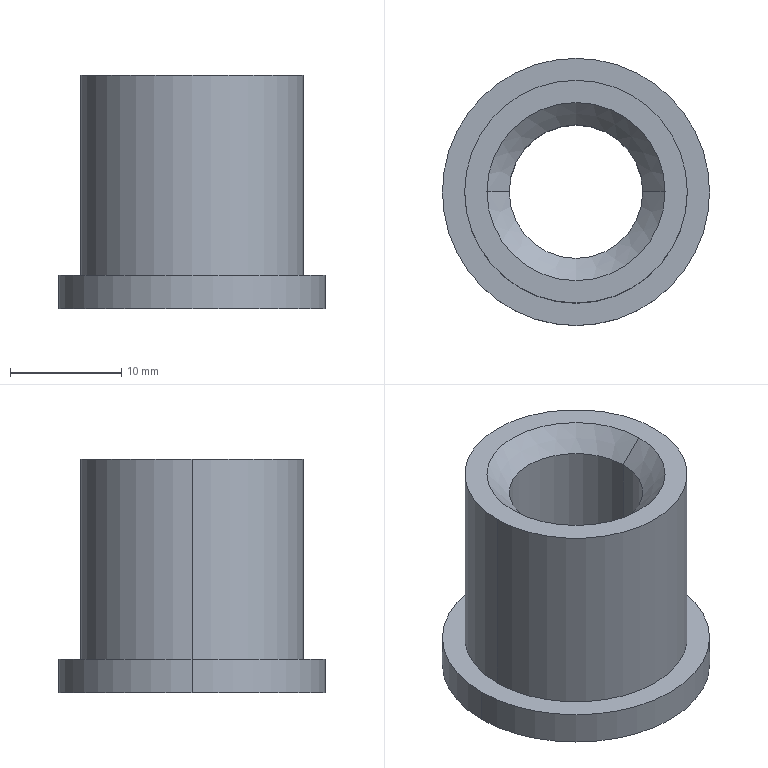Part | SolidWorks | features ICE 2, Chamfer 1, Extrusion 1 | 1 solid | 11 faces | box 24 x 24 x 21 mm | volume 4553 mm3 | cylinder 6 | plane 3 | cone 2 | commonest cylinder face diameters 12 x2 20 x2 24 x2
STEP:
#1=CARTESIAN_POINT('',(-6.,0.,19.));
#2=VERTEX_POINT('',#1);
#3=CARTESIAN_POINT('',(6.,0.,19.));
#4=VERTEX_POINT('',#3);
#5=CARTESIAN_POINT('',(0.,0.,19.));
#6=DIRECTION('',(0.,0.,1.));
#7=DIRECTION('',(1.,0.,0.));
#8=AXIS2_PLACEMENT_3D('',#5,#6,#7);
#9=CIRCLE('',#8,6.);
#10=EDGE_CURVE('',#2,#4,#9,.T.);
#11=ORIENTED_EDGE('',*,*,#10,.F.);
#12=CARTESIAN_POINT('',(-8.,0.,21.));
#13=VERTEX_POINT('',#12);
#14=CARTESIAN_POINT('',(-6.,0.,19.));
#15=DIRECTION('',(-0.7071,0.,0.7071));
#16=VECTOR('',#15,1000.);
#17=LINE('',#14,#16);
#18=EDGE_CURVE('',#2,#13,#17,.T.);
#19=ORIENTED_EDGE('',*,*,#18,.T.);
#20=CARTESIAN_POINT('',(8.,0.,21.));
#21=VERTEX_POINT('',#20);
#22=CARTESIAN_POINT('',(0.,0.,21.));
#23=DIRECTION('',(0.,0.,-1.));
#24=DIRECTION('',(1.,0.,0.));
#25=AXIS2_PLACEMENT_3D('',#22,#23,#24);
#26=CIRCLE('',#25,8.);
#27=EDGE_CURVE('',#21,#13,#26,.T.);
#28=ORIENTED_EDGE('',*,*,#27,.F.);
#29=CARTESIAN_POINT('',(6.,0.,19.));
#30=DIRECTION('',(0.7071,0.,0.7071));
#31=VECTOR('',#30,1000.);
#32=LINE('',#29,#31);
#33=EDGE_CURVE('',#4,#21,#32,.T.);
#34=ORIENTED_EDGE('',*,*,#33,.F.);
#35=EDGE_LOOP('',(#11,#19,#28,#34));
#36=FACE_OUTER_BOUND('',#35,.T.);
#37=CARTESIAN_POINT('',(0.,0.,19.));
#38=DIRECTION('',(0.,0.,1.));
#39=DIRECTION('',(1.,0.,0.));
#40=AXIS2_PLACEMENT_3D('',#37,#38,#39);
#41=CONICAL_SURFACE('',#40,6.,0.7854);
#42=ADVANCED_FACE('',(#36),#41,.F.);
#43=CARTESIAN_POINT('',(-6.,0.,0.));
#44=VERTEX_POINT('',#43);
#45=CARTESIAN_POINT('',(6.,0.,0.));
#46=VERTEX_POINT('',#45);
#47=CARTESIAN_POINT('',(0.,0.,0.));
#48=DIRECTION('',(0.,0.,1.));
#49=DIRECTION('',(1.,0.,0.));
#50=AXIS2_PLACEMENT_3D('',#47,#48,#49);
#51=CIRCLE('',#50,6.);
#52=EDGE_CURVE('',#44,#46,#51,.T.);
#53=ORIENTED_EDGE('',*,*,#52,.F.);
#54=CARTESIAN_POINT('',(-6.,0.,-5.));
#55=DIRECTION('',(0.,0.,1.));
#56=VECTOR('',#55,1000.);
#57=LINE('',#54,#56);
#58=EDGE_CURVE('',#44,#2,#57,.T.);
#59=ORIENTED_EDGE('',*,*,#58,.T.);
#60=ORIENTED_EDGE('',*,*,#10,.T.);
#61=CARTESIAN_POINT('',(6.,0.,-5.));
#62=DIRECTION('',(0.,0.,1.));
#63=VECTOR('',#62,1000.);
#64=LINE('',#61,#63);
#65=EDGE_CURVE('',#46,#4,#64,.T.);
#66=ORIENTED_EDGE('',*,*,#65,.F.);
#67=EDGE_LOOP('',(#53,#59,#60,#66));
#68=FACE_OUTER_BOUND('',#67,.T.);
#69=CARTESIAN_POINT('',(0.,0.,-5.));
#70=DIRECTION('',(0.,0.,1.));
#71=DIRECTION('',(1.,0.,0.));
#72=AXIS2_PLACEMENT_3D('',#69,#70,#71);
#73=CYLINDRICAL_SURFACE('',#72,6.);
#74=ADVANCED_FACE('',(#68),#73,.F.);
#75=CARTESIAN_POINT('',(10.,0.,21.));
#76=VERTEX_POINT('',#75);
#77=CARTESIAN_POINT('',(-10.,0.,21.));
#78=VERTEX_POINT('',#77);
#79=CARTESIAN_POINT('',(0.,0.,21.));
#80=DIRECTION('',(0.,0.,1.));
#81=DIRECTION('',(1.,0.,0.));
#82=AXIS2_PLACEMENT_3D('',#79,#80,#81);
#83=CIRCLE('',#82,10.);
#84=EDGE_CURVE('',#76,#78,#83,.T.);
#85=ORIENTED_EDGE('',*,*,#84,.F.);
#86=CARTESIAN_POINT('',(10.,0.,3.));
#87=VERTEX_POINT('',#86);
#88=CARTESIAN_POINT('',(10.,0.,21.));
#89=DIRECTION('',(0.,0.,-1.));
#90=VECTOR('',#89,1000.);
#91=LINE('',#88,#90);
#92=EDGE_CURVE('',#76,#87,#91,.T.);
#93=ORIENTED_EDGE('',*,*,#92,.T.);
#94=CARTESIAN_POINT('',(-10.,0.,3.));
#95=VERTEX_POINT('',#94);
#96=CARTESIAN_POINT('',(0.,0.,3.));
#97=DIRECTION('',(0.,0.,1.));
#98=DIRECTION('',(1.,0.,0.));
#99=AXIS2_PLACEMENT_3D('',#96,#97,#98);
#100=CIRCLE('',#99,10.);
#101=EDGE_CURVE('',#87,#95,#100,.T.);
#102=ORIENTED_EDGE('',*,*,#101,.T.);
#103=CARTESIAN_POINT('',(-10.,0.,21.));
#104=DIRECTION('',(0.,0.,-1.));
#105=VECTOR('',#104,1000.);
#106=LINE('',#103,#105);
#107=EDGE_CURVE('',#78,#95,#106,.T.);
#108=ORIENTED_EDGE('',*,*,#107,.F.);
#109=EDGE_LOOP('',(#85,#93,#102,#108));
#110=FACE_OUTER_BOUND('',#109,.T.);
#111=CARTESIAN_POINT('',(0.,0.,21.));
#112=DIRECTION('',(0.,0.,-1.));
#113=DIRECTION('',(-1.,0.,0.));
#114=AXIS2_PLACEMENT_3D('',#111,#112,#113);
#115=CYLINDRICAL_SURFACE('',#114,10.);
#116=ADVANCED_FACE('',(#110),#115,.T.);
#117=CARTESIAN_POINT('',(12.,0.,3.));
#118=VERTEX_POINT('',#117);
#119=CARTESIAN_POINT('',(-12.,0.,3.));
#120=VERTEX_POINT('',#119);
#121=CARTESIAN_POINT('',(0.,0.,3.));
#122=DIRECTION('',(0.,0.,1.));
#123=DIRECTION('',(1.,0.,0.));
#124=AXIS2_PLACEMENT_3D('',#121,#122,#123);
#125=CIRCLE('',#124,12.);
#126=EDGE_CURVE('',#118,#120,#125,.T.);
#127=ORIENTED_EDGE('',*,*,#126,.F.);
#128=CARTESIAN_POINT('',(12.,0.,0.));
#129=VERTEX_POINT('',#128);
#130=CARTESIAN_POINT('',(12.,0.,3.));
#131=DIRECTION('',(0.,0.,-1.));
#132=VECTOR('',#131,1000.);
#133=LINE('',#130,#132);
#134=EDGE_CURVE('',#118,#129,#133,.T.);
#135=ORIENTED_EDGE('',*,*,#134,.T.);
#136=CARTESIAN_POINT('',(-12.,0.,0.));
#137=VERTEX_POINT('',#136);
#138=CARTESIAN_POINT('',(0.,0.,0.));
#139=DIRECTION('',(0.,0.,1.));
#140=DIRECTION('',(1.,0.,0.));
#141=AXIS2_PLACEMENT_3D('',#138,#139,#140);
#142=CIRCLE('',#141,12.);
#143=EDGE_CURVE('',#129,#137,#142,.T.);
#144=ORIENTED_EDGE('',*,*,#143,.T.);
#145=CARTESIAN_POINT('',(-12.,0.,3.));
#146=DIRECTION('',(0.,0.,-1.));
#147=VECTOR('',#146,1000.);
#148=LINE('',#145,#147);
#149=EDGE_CURVE('',#120,#137,#148,.T.);
#150=ORIENTED_EDGE('',*,*,#149,.F.);
#151=EDGE_LOOP('',(#127,#135,#144,#150));
#152=FACE_OUTER_BOUND('',#151,.T.);
#153=CARTESIAN_POINT('',(0.,0.,3.));
#154=DIRECTION('',(0.,0.,-1.));
#155=DIRECTION('',(-1.,0.,0.));
#156=AXIS2_PLACEMENT_3D('',#153,#154,#155);
#157=CYLINDRICAL_SURFACE('',#156,12.);
#158=ADVANCED_FACE('',(#152),#157,.T.);
#159=CARTESIAN_POINT('',(0.,0.,3.));
#160=DIRECTION('',(0.,0.,1.));
#161=DIRECTION('',(1.,0.,0.));
#162=AXIS2_PLACEMENT_3D('',#159,#160,#161);
#163=CIRCLE('',#162,12.);
#164=EDGE_CURVE('',#120,#118,#163,.T.);
#165=ORIENTED_EDGE('',*,*,#164,.T.);
#166=ORIENTED_EDGE('',*,*,#126,.T.);
#167=EDGE_LOOP('',(#165,#166));
#168=FACE_OUTER_BOUND('',#167,.T.);
#169=CARTESIAN_POINT('',(0.,0.,3.));
#170=DIRECTION('',(0.,0.,1.));
#171=DIRECTION('',(1.,0.,0.));
#172=AXIS2_PLACEMENT_3D('',#169,#170,#171);
#173=CIRCLE('',#172,10.);
#174=EDGE_CURVE('',#95,#87,#173,.T.);
#175=ORIENTED_EDGE('',*,*,#174,.F.);
#176=ORIENTED_EDGE('',*,*,#101,.F.);
#177=EDGE_LOOP('',(#175,#176));
#178=FACE_BOUND('',#177,.T.);
#179=CARTESIAN_POINT('',(0.,0.,3.));
#180=DIRECTION('',(0.,0.,1.));
#181=DIRECTION('',(1.,0.,0.));
#182=AXIS2_PLACEMENT_3D('',#179,#180,#181);
#183=PLANE('',#182);
#184=ADVANCED_FACE('',(#168,#178),#183,.T.);
#185=ORIENTED_EDGE('',*,*,#134,.F.);
#186=ORIENTED_EDGE('',*,*,#164,.F.);
#187=ORIENTED_EDGE('',*,*,#149,.T.);
#188=CARTESIAN_POINT('',(0.,0.,0.));
#189=DIRECTION('',(0.,0.,1.));
#190=DIRECTION('',(1.,0.,0.));
#191=AXIS2_PLACEMENT_3D('',#188,#189,#190);
#192=CIRCLE('',#191,12.);
#193=EDGE_CURVE('',#137,#129,#192,.T.);
#194=ORIENTED_EDGE('',*,*,#193,.T.);
#195=EDGE_LOOP('',(#185,#186,#187,#194));
#196=FACE_OUTER_BOUND('',#195,.T.);
#197=CARTESIAN_POINT('',(0.,0.,3.));
#198=DIRECTION('',(0.,0.,-1.));
#199=DIRECTION('',(-1.,0.,0.));
#200=AXIS2_PLACEMENT_3D('',#197,#198,#199);
#201=CYLINDRICAL_SURFACE('',#200,12.);
#202=ADVANCED_FACE('',(#196),#201,.T.);
#203=CARTESIAN_POINT('',(0.,0.,0.));
#204=DIRECTION('',(0.,0.,1.));
#205=DIRECTION('',(1.,0.,0.));
#206=AXIS2_PLACEMENT_3D('',#203,#204,#205);
#207=CIRCLE('',#206,6.);
#208=EDGE_CURVE('',#46,#44,#207,.T.);
#209=ORIENTED_EDGE('',*,*,#208,.T.);
#210=ORIENTED_EDGE('',*,*,#52,.T.);
#211=EDGE_LOOP('',(#209,#210));
#212=FACE_BOUND('',#211,.T.);
#213=ORIENTED_EDGE('',*,*,#193,.F.);
#214=ORIENTED_EDGE('',*,*,#143,.F.);
#215=EDGE_LOOP('',(#213,#214));
#216=FACE_OUTER_BOUND('',#215,.T.);
#217=CARTESIAN_POINT('',(0.,0.,0.));
#218=DIRECTION('',(0.,0.,1.));
#219=DIRECTION('',(1.,0.,0.));
#220=AXIS2_PLACEMENT_3D('',#217,#218,#219);
#221=PLANE('',#220);
#222=ADVANCED_FACE('',(#212,#216),#221,.F.);
#223=ORIENTED_EDGE('',*,*,#92,.F.);
#224=CARTESIAN_POINT('',(0.,0.,21.));
#225=DIRECTION('',(0.,0.,1.));
#226=DIRECTION('',(1.,0.,0.));
#227=AXIS2_PLACEMENT_3D('',#224,#225,#226);
#228=CIRCLE('',#227,10.);
#229=EDGE_CURVE('',#78,#76,#228,.T.);
#230=ORIENTED_EDGE('',*,*,#229,.F.);
#231=ORIENTED_EDGE('',*,*,#107,.T.);
#232=ORIENTED_EDGE('',*,*,#174,.T.);
#233=EDGE_LOOP('',(#223,#230,#231,#232));
#234=FACE_OUTER_BOUND('',#233,.T.);
#235=CARTESIAN_POINT('',(0.,0.,21.));
#236=DIRECTION('',(0.,0.,-1.));
#237=DIRECTION('',(-1.,0.,0.));
#238=AXIS2_PLACEMENT_3D('',#235,#236,#237);
#239=CYLINDRICAL_SURFACE('',#238,10.);
#240=ADVANCED_FACE('',(#234),#239,.T.);
#241=ORIENTED_EDGE('',*,*,#27,.T.);
#242=CARTESIAN_POINT('',(0.,0.,21.));
#243=DIRECTION('',(0.,0.,-1.));
#244=DIRECTION('',(1.,0.,0.));
#245=AXIS2_PLACEMENT_3D('',#242,#243,#244);
#246=CIRCLE('',#245,8.);
#247=EDGE_CURVE('',#13,#21,#246,.T.);
#248=ORIENTED_EDGE('',*,*,#247,.T.);
#249=EDGE_LOOP('',(#241,#248));
#250=FACE_BOUND('',#249,.T.);
#251=ORIENTED_EDGE('',*,*,#229,.T.);
#252=ORIENTED_EDGE('',*,*,#84,.T.);
#253=EDGE_LOOP('',(#251,#252));
#254=FACE_OUTER_BOUND('',#253,.T.);
#255=CARTESIAN_POINT('',(0.,0.,21.));
#256=DIRECTION('',(0.,0.,1.));
#257=DIRECTION('',(1.,0.,0.));
#258=AXIS2_PLACEMENT_3D('',#255,#256,#257);
#259=PLANE('',#258);
#260=ADVANCED_FACE('',(#250,#254),#259,.T.);
#261=ORIENTED_EDGE('',*,*,#58,.F.);
#262=ORIENTED_EDGE('',*,*,#208,.F.);
#263=ORIENTED_EDGE('',*,*,#65,.T.);
#264=CARTESIAN_POINT('',(0.,0.,19.));
#265=DIRECTION('',(0.,0.,1.));
#266=DIRECTION('',(1.,0.,0.));
#267=AXIS2_PLACEMENT_3D('',#264,#265,#266);
#268=CIRCLE('',#267,6.);
#269=EDGE_CURVE('',#4,#2,#268,.T.);
#270=ORIENTED_EDGE('',*,*,#269,.T.);
#271=EDGE_LOOP('',(#261,#262,#263,#270));
#272=FACE_OUTER_BOUND('',#271,.T.);
#273=CARTESIAN_POINT('',(0.,0.,-5.));
#274=DIRECTION('',(0.,0.,1.));
#275=DIRECTION('',(1.,0.,0.));
#276=AXIS2_PLACEMENT_3D('',#273,#274,#275);
#277=CYLINDRICAL_SURFACE('',#276,6.);
#278=ADVANCED_FACE('',(#272),#277,.F.);
#279=ORIENTED_EDGE('',*,*,#18,.F.);
#280=ORIENTED_EDGE('',*,*,#269,.F.);
#281=ORIENTED_EDGE('',*,*,#33,.T.);
#282=ORIENTED_EDGE('',*,*,#247,.F.);
#283=EDGE_LOOP('',(#279,#280,#281,#282));
#284=FACE_OUTER_BOUND('',#283,.T.);
#285=CARTESIAN_POINT('',(0.,0.,19.));
#286=DIRECTION('',(0.,0.,1.));
#287=DIRECTION('',(1.,0.,0.));
#288=AXIS2_PLACEMENT_3D('',#285,#286,#287);
#289=CONICAL_SURFACE('',#288,6.,0.7854);
#290=ADVANCED_FACE('',(#284),#289,.F.);
#291=CLOSED_SHELL('',(#42,#74,#116,#158,#184,#202,#222,#240,#260,#278,#290));
#292=MANIFOLD_SOLID_BREP('',#291);
#293=CARTESIAN_POINT('',(0.,0.,0.));
#294=DIRECTION('',(0.,0.,1.));
#295=DIRECTION('',(1.,0.,0.));
#296=AXIS2_PLACEMENT_3D('',#293,#294,#295);
#297=(LENGTH_UNIT()NAMED_UNIT(*)SI_UNIT(.MILLI.,.METRE.));
#298=UNCERTAINTY_MEASURE_WITH_UNIT(LENGTH_MEASURE(0.00001),#297,'','');
#299=(NAMED_UNIT(*)PLANE_ANGLE_UNIT()SI_UNIT($,.RADIAN.));
#300=(NAMED_UNIT(*)SI_UNIT($,.STERADIAN.)SOLID_ANGLE_UNIT());
#301=(GEOMETRIC_REPRESENTATION_CONTEXT(3)GLOBAL_UNCERTAINTY_ASSIGNED_CONTEXT((#298))GLOBAL_UNIT_ASSIGNED_CONTEXT((#297,#299,#300))REPRESENTATION_CONTEXT('',''));
#302=ADVANCED_BREP_SHAPE_REPRESENTATION('',(#292,#296),#301);